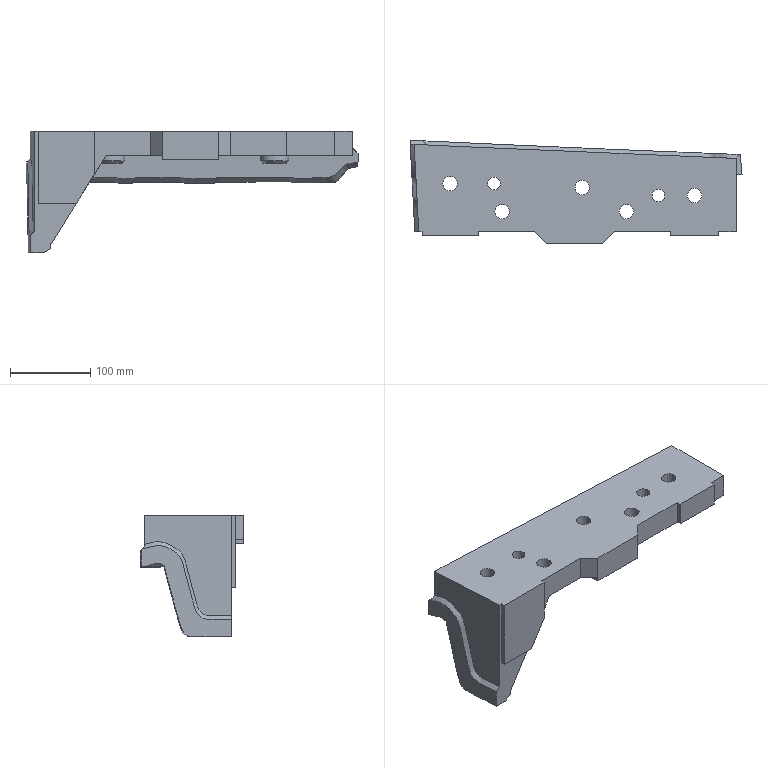Part | NX | features solid 2 | 1 solid | 68 faces | box 414.193 x 129.147 x 152.075 mm | volume 1839935 mm3 | plane 35 | spline 17 | cylinder 14 | cone 2 | commonest cylinder face diameters 18 x5 26 x5 16 x2 36 x2